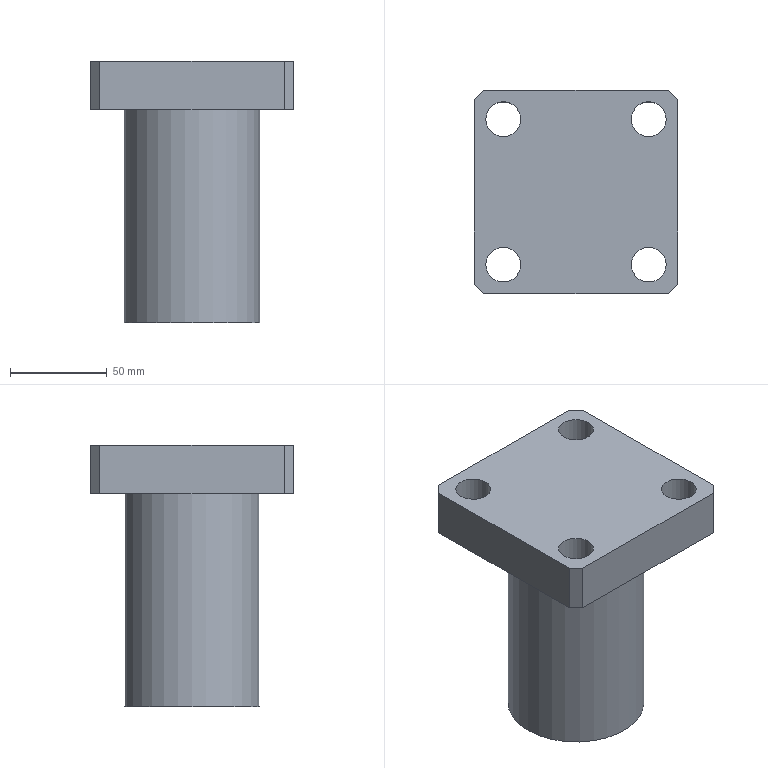Part | NX | features solid 2 | 1 solid | 16 faces | box 105 x 105 x 135 mm | volume 672258 mm3 | plane 11 | cylinder 5 | commonest cylinder face diameters 18 x4 70 x1
STEP:
#1=CARTESIAN_POINT('',(-237.5,207.5,100.));
#2=VERTEX_POINT('',#1);
#3=CARTESIAN_POINT('',(-237.5,112.5,100.));
#4=VERTEX_POINT('',#3);
#5=CARTESIAN_POINT('',(-237.5,210.,100.));
#6=DIRECTION('',(0.,-1.,0.));
#7=VECTOR('',#6,1000.);
#8=LINE('',#5,#7);
#9=EDGE_CURVE('',#2,#4,#8,.T.);
#10=ORIENTED_EDGE('',*,*,#9,.F.);
#11=CARTESIAN_POINT('',(-237.5,207.5,75.));
#12=VERTEX_POINT('',#11);
#13=CARTESIAN_POINT('',(-237.5,207.5,90.));
#14=DIRECTION('',(0.,0.,-1.));
#15=VECTOR('',#14,1000.);
#16=LINE('',#13,#15);
#17=EDGE_CURVE('',#2,#12,#16,.T.);
#18=ORIENTED_EDGE('',*,*,#17,.T.);
#19=CARTESIAN_POINT('',(-237.5,112.5,75.));
#20=VERTEX_POINT('',#19);
#21=CARTESIAN_POINT('',(-237.5,210.,75.));
#22=DIRECTION('',(0.,-1.,0.));
#23=VECTOR('',#22,1000.);
#24=LINE('',#21,#23);
#25=EDGE_CURVE('',#12,#20,#24,.T.);
#26=ORIENTED_EDGE('',*,*,#25,.T.);
#27=CARTESIAN_POINT('',(-237.5,112.5,90.));
#28=DIRECTION('',(0.,0.,1.));
#29=VECTOR('',#28,1000.);
#30=LINE('',#27,#29);
#31=EDGE_CURVE('',#20,#4,#30,.T.);
#32=ORIENTED_EDGE('',*,*,#31,.T.);
#33=EDGE_LOOP('',(#10,#18,#26,#32));
#34=FACE_BOUND('',#33,.T.);
#35=CARTESIAN_POINT('',(-237.5,210.,90.));
#36=DIRECTION('',(1.,0.,0.));
#37=DIRECTION('',(0.,0.,-1.));
#38=AXIS2_PLACEMENT_3D('',#35,#36,#37);
#39=PLANE('',#38);
#40=ADVANCED_FACE('',(#34),#39,.F.);
#41=CARTESIAN_POINT('',(-132.5,207.5,100.));
#42=VERTEX_POINT('',#41);
#43=CARTESIAN_POINT('',(-132.5,112.5,100.));
#44=VERTEX_POINT('',#43);
#45=CARTESIAN_POINT('',(-132.5,210.,100.));
#46=DIRECTION('',(0.,-1.,0.));
#47=VECTOR('',#46,1000.);
#48=LINE('',#45,#47);
#49=EDGE_CURVE('',#42,#44,#48,.T.);
#50=ORIENTED_EDGE('',*,*,#49,.T.);
#51=CARTESIAN_POINT('',(-132.5,112.5,75.));
#52=VERTEX_POINT('',#51);
#53=CARTESIAN_POINT('',(-132.5,112.5,75.));
#54=DIRECTION('',(0.,0.,-1.));
#55=VECTOR('',#54,1000.);
#56=LINE('',#53,#55);
#57=EDGE_CURVE('',#44,#52,#56,.T.);
#58=ORIENTED_EDGE('',*,*,#57,.T.);
#59=CARTESIAN_POINT('',(-132.5,207.5,75.));
#60=VERTEX_POINT('',#59);
#61=CARTESIAN_POINT('',(-132.5,210.,75.));
#62=DIRECTION('',(0.,-1.,0.));
#63=VECTOR('',#62,1000.);
#64=LINE('',#61,#63);
#65=EDGE_CURVE('',#60,#52,#64,.T.);
#66=ORIENTED_EDGE('',*,*,#65,.F.);
#67=CARTESIAN_POINT('',(-132.5,207.5,100.));
#68=DIRECTION('',(0.,0.,1.));
#69=VECTOR('',#68,1000.);
#70=LINE('',#67,#69);
#71=EDGE_CURVE('',#60,#42,#70,.T.);
#72=ORIENTED_EDGE('',*,*,#71,.T.);
#73=EDGE_LOOP('',(#50,#58,#66,#72));
#74=FACE_BOUND('',#73,.T.);
#75=CARTESIAN_POINT('',(-132.5,210.,90.));
#76=DIRECTION('',(1.,0.,0.));
#77=DIRECTION('',(0.,0.,-1.));
#78=AXIS2_PLACEMENT_3D('',#75,#76,#77);
#79=PLANE('',#78);
#80=ADVANCED_FACE('',(#74),#79,.T.);
#81=CARTESIAN_POINT('',(-137.5,212.5,100.));
#82=VERTEX_POINT('',#81);
#83=CARTESIAN_POINT('',(-232.5,212.5,100.));
#84=VERTEX_POINT('',#83);
#85=CARTESIAN_POINT('',(-185.,212.5,100.));
#86=DIRECTION('',(-1.,0.,0.));
#87=VECTOR('',#86,1000.);
#88=LINE('',#85,#87);
#89=EDGE_CURVE('',#82,#84,#88,.T.);
#90=ORIENTED_EDGE('',*,*,#89,.F.);
#91=CARTESIAN_POINT('',(-137.5,212.5,75.));
#92=VERTEX_POINT('',#91);
#93=CARTESIAN_POINT('',(-137.5,212.5,75.));
#94=DIRECTION('',(0.,0.,-1.));
#95=VECTOR('',#94,1000.);
#96=LINE('',#93,#95);
#97=EDGE_CURVE('',#82,#92,#96,.T.);
#98=ORIENTED_EDGE('',*,*,#97,.T.);
#99=CARTESIAN_POINT('',(-232.5,212.5,75.));
#100=VERTEX_POINT('',#99);
#101=CARTESIAN_POINT('',(-185.,212.5,75.));
#102=DIRECTION('',(-1.,0.,0.));
#103=VECTOR('',#102,1000.);
#104=LINE('',#101,#103);
#105=EDGE_CURVE('',#92,#100,#104,.T.);
#106=ORIENTED_EDGE('',*,*,#105,.T.);
#107=CARTESIAN_POINT('',(-232.5,212.5,90.));
#108=DIRECTION('',(0.,0.,1.));
#109=VECTOR('',#108,1000.);
#110=LINE('',#107,#109);
#111=EDGE_CURVE('',#100,#84,#110,.T.);
#112=ORIENTED_EDGE('',*,*,#111,.T.);
#113=EDGE_LOOP('',(#90,#98,#106,#112));
#114=FACE_BOUND('',#113,.T.);
#115=CARTESIAN_POINT('',(-185.,212.5,90.));
#116=DIRECTION('',(0.,-1.,0.));
#117=DIRECTION('',(0.,0.,-1.));
#118=AXIS2_PLACEMENT_3D('',#115,#116,#117);
#119=PLANE('',#118);
#120=ADVANCED_FACE('',(#114),#119,.F.);
#121=CARTESIAN_POINT('',(-232.5,107.5,75.));
#122=VERTEX_POINT('',#121);
#123=CARTESIAN_POINT('',(-137.5,107.5,75.));
#124=VERTEX_POINT('',#123);
#125=CARTESIAN_POINT('',(-185.,107.5,75.));
#126=DIRECTION('',(-1.,0.,0.));
#127=VECTOR('',#126,1000.);
#128=LINE('',#125,#127);
#129=EDGE_CURVE('',#122,#124,#128,.F.);
#130=ORIENTED_EDGE('',*,*,#129,.T.);
#131=CARTESIAN_POINT('',(-137.5,107.5,100.));
#132=VERTEX_POINT('',#131);
#133=CARTESIAN_POINT('',(-137.5,107.5,100.));
#134=DIRECTION('',(0.,0.,-1.));
#135=VECTOR('',#134,1000.);
#136=LINE('',#133,#135);
#137=EDGE_CURVE('',#124,#132,#136,.F.);
#138=ORIENTED_EDGE('',*,*,#137,.T.);
#139=CARTESIAN_POINT('',(-232.5,107.5,100.));
#140=VERTEX_POINT('',#139);
#141=CARTESIAN_POINT('',(-185.,107.5,100.));
#142=DIRECTION('',(1.,0.,0.));
#143=VECTOR('',#142,1000.);
#144=LINE('',#141,#143);
#145=EDGE_CURVE('',#132,#140,#144,.F.);
#146=ORIENTED_EDGE('',*,*,#145,.T.);
#147=CARTESIAN_POINT('',(-232.5,107.5,90.));
#148=DIRECTION('',(0.,0.,1.));
#149=VECTOR('',#148,1000.);
#150=LINE('',#147,#149);
#151=EDGE_CURVE('',#140,#122,#150,.F.);
#152=ORIENTED_EDGE('',*,*,#151,.T.);
#153=EDGE_LOOP('',(#130,#138,#146,#152));
#154=FACE_BOUND('',#153,.T.);
#155=CARTESIAN_POINT('',(-185.,107.5,90.));
#156=DIRECTION('',(0.,-1.,0.));
#157=DIRECTION('',(0.,0.,-1.));
#158=AXIS2_PLACEMENT_3D('',#155,#156,#157);
#159=PLANE('',#158);
#160=ADVANCED_FACE('',(#154),#159,.T.);
#161=CARTESIAN_POINT('',(-138.5,122.5,75.));
#162=VERTEX_POINT('',#161);
#163=CARTESIAN_POINT('',(-147.5,122.5,75.));
#164=DIRECTION('',(0.,0.,1.));
#165=DIRECTION('',(1.,0.,0.));
#166=AXIS2_PLACEMENT_3D('',#163,#164,#165);
#167=CIRCLE('',#166,9.);
#168=EDGE_CURVE('',#162,#162,#167,.F.);
#169=ORIENTED_EDGE('',*,*,#168,.T.);
#170=EDGE_LOOP('',(#169));
#171=FACE_BOUND('',#170,.T.);
#172=CARTESIAN_POINT('',(-138.5,122.5,100.));
#173=VERTEX_POINT('',#172);
#174=CARTESIAN_POINT('',(-147.5,122.5,100.));
#175=DIRECTION('',(0.,0.,1.));
#176=DIRECTION('',(1.,0.,0.));
#177=AXIS2_PLACEMENT_3D('',#174,#175,#176);
#178=CIRCLE('',#177,9.);
#179=EDGE_CURVE('',#173,#173,#178,.T.);
#180=ORIENTED_EDGE('',*,*,#179,.T.);
#181=EDGE_LOOP('',(#180));
#182=FACE_BOUND('',#181,.T.);
#183=CARTESIAN_POINT('',(-147.5,122.5,65.));
#184=DIRECTION('',(0.,0.,1.));
#185=DIRECTION('',(1.,0.,0.));
#186=AXIS2_PLACEMENT_3D('',#183,#184,#185);
#187=CYLINDRICAL_SURFACE('',#186,9.);
#188=ADVANCED_FACE('',(#171,#182),#187,.F.);
#189=CARTESIAN_POINT('',(-213.5,122.5,75.));
#190=VERTEX_POINT('',#189);
#191=CARTESIAN_POINT('',(-222.5,122.5,75.));
#192=DIRECTION('',(0.,0.,1.));
#193=DIRECTION('',(1.,0.,0.));
#194=AXIS2_PLACEMENT_3D('',#191,#192,#193);
#195=CIRCLE('',#194,9.);
#196=EDGE_CURVE('',#190,#190,#195,.F.);
#197=ORIENTED_EDGE('',*,*,#196,.T.);
#198=EDGE_LOOP('',(#197));
#199=FACE_BOUND('',#198,.T.);
#200=CARTESIAN_POINT('',(-213.5,122.5,100.));
#201=VERTEX_POINT('',#200);
#202=CARTESIAN_POINT('',(-222.5,122.5,100.));
#203=DIRECTION('',(0.,0.,1.));
#204=DIRECTION('',(1.,0.,0.));
#205=AXIS2_PLACEMENT_3D('',#202,#203,#204);
#206=CIRCLE('',#205,9.);
#207=EDGE_CURVE('',#201,#201,#206,.T.);
#208=ORIENTED_EDGE('',*,*,#207,.T.);
#209=EDGE_LOOP('',(#208));
#210=FACE_BOUND('',#209,.T.);
#211=CARTESIAN_POINT('',(-222.5,122.5,65.));
#212=DIRECTION('',(0.,0.,1.));
#213=DIRECTION('',(1.,0.,0.));
#214=AXIS2_PLACEMENT_3D('',#211,#212,#213);
#215=CYLINDRICAL_SURFACE('',#214,9.);
#216=ADVANCED_FACE('',(#199,#210),#215,.F.);
#217=CARTESIAN_POINT('',(-213.5,197.5,75.));
#218=VERTEX_POINT('',#217);
#219=CARTESIAN_POINT('',(-222.5,197.5,75.));
#220=DIRECTION('',(0.,0.,1.));
#221=DIRECTION('',(1.,0.,0.));
#222=AXIS2_PLACEMENT_3D('',#219,#220,#221);
#223=CIRCLE('',#222,9.);
#224=EDGE_CURVE('',#218,#218,#223,.F.);
#225=ORIENTED_EDGE('',*,*,#224,.T.);
#226=EDGE_LOOP('',(#225));
#227=FACE_BOUND('',#226,.T.);
#228=CARTESIAN_POINT('',(-213.5,197.5,100.));
#229=VERTEX_POINT('',#228);
#230=CARTESIAN_POINT('',(-222.5,197.5,100.));
#231=DIRECTION('',(0.,0.,1.));
#232=DIRECTION('',(1.,0.,0.));
#233=AXIS2_PLACEMENT_3D('',#230,#231,#232);
#234=CIRCLE('',#233,9.);
#235=EDGE_CURVE('',#229,#229,#234,.T.);
#236=ORIENTED_EDGE('',*,*,#235,.T.);
#237=EDGE_LOOP('',(#236));
#238=FACE_BOUND('',#237,.T.);
#239=CARTESIAN_POINT('',(-222.5,197.5,65.));
#240=DIRECTION('',(0.,0.,1.));
#241=DIRECTION('',(1.,0.,0.));
#242=AXIS2_PLACEMENT_3D('',#239,#240,#241);
#243=CYLINDRICAL_SURFACE('',#242,9.);
#244=ADVANCED_FACE('',(#227,#238),#243,.F.);
#245=CARTESIAN_POINT('',(-138.5,197.5,100.));
#246=VERTEX_POINT('',#245);
#247=CARTESIAN_POINT('',(-147.5,197.5,100.));
#248=DIRECTION('',(0.,0.,1.));
#249=DIRECTION('',(1.,0.,0.));
#250=AXIS2_PLACEMENT_3D('',#247,#248,#249);
#251=CIRCLE('',#250,9.);
#252=EDGE_CURVE('',#246,#246,#251,.T.);
#253=ORIENTED_EDGE('',*,*,#252,.F.);
#254=EDGE_LOOP('',(#253));
#255=FACE_BOUND('',#254,.T.);
#256=ORIENTED_EDGE('',*,*,#235,.F.);
#257=EDGE_LOOP('',(#256));
#258=FACE_BOUND('',#257,.T.);
#259=ORIENTED_EDGE('',*,*,#207,.F.);
#260=EDGE_LOOP('',(#259));
#261=FACE_BOUND('',#260,.T.);
#262=ORIENTED_EDGE('',*,*,#179,.F.);
#263=EDGE_LOOP('',(#262));
#264=FACE_BOUND('',#263,.T.);
#265=ORIENTED_EDGE('',*,*,#145,.F.);
#266=CARTESIAN_POINT('',(-135.,110.,100.));
#267=DIRECTION('',(-0.7071,-0.7071,0.));
#268=VECTOR('',#267,1000.);
#269=LINE('',#266,#268);
#270=EDGE_CURVE('',#132,#44,#269,.F.);
#271=ORIENTED_EDGE('',*,*,#270,.T.);
#272=ORIENTED_EDGE('',*,*,#49,.F.);
#273=CARTESIAN_POINT('',(-135.,210.,100.));
#274=DIRECTION('',(-0.7071,0.7071,0.));
#275=VECTOR('',#274,1000.);
#276=LINE('',#273,#275);
#277=EDGE_CURVE('',#42,#82,#276,.T.);
#278=ORIENTED_EDGE('',*,*,#277,.T.);
#279=ORIENTED_EDGE('',*,*,#89,.T.);
#280=CARTESIAN_POINT('',(-235.,210.,100.));
#281=DIRECTION('',(0.7071,0.7071,0.));
#282=VECTOR('',#281,1000.);
#283=LINE('',#280,#282);
#284=EDGE_CURVE('',#84,#2,#283,.F.);
#285=ORIENTED_EDGE('',*,*,#284,.T.);
#286=ORIENTED_EDGE('',*,*,#9,.T.);
#287=CARTESIAN_POINT('',(-235.,110.,100.));
#288=DIRECTION('',(0.7071,-0.7071,0.));
#289=VECTOR('',#288,1000.);
#290=LINE('',#287,#289);
#291=EDGE_CURVE('',#4,#140,#290,.T.);
#292=ORIENTED_EDGE('',*,*,#291,.T.);
#293=EDGE_LOOP('',(#265,#271,#272,#278,#279,#285,#286,#292));
#294=FACE_BOUND('',#293,.T.);
#295=CARTESIAN_POINT('',(-185.,160.,100.));
#296=DIRECTION('',(0.,0.,1.));
#297=DIRECTION('',(1.,0.,0.));
#298=AXIS2_PLACEMENT_3D('',#295,#296,#297);
#299=PLANE('',#298);
#300=ADVANCED_FACE('',(#255,#258,#261,#264,#294),#299,.T.);
#301=CARTESIAN_POINT('',(-138.5,197.5,75.));
#302=VERTEX_POINT('',#301);
#303=CARTESIAN_POINT('',(-147.5,197.5,75.));
#304=DIRECTION('',(0.,0.,1.));
#305=DIRECTION('',(1.,0.,0.));
#306=AXIS2_PLACEMENT_3D('',#303,#304,#305);
#307=CIRCLE('',#306,9.);
#308=EDGE_CURVE('',#302,#302,#307,.F.);
#309=ORIENTED_EDGE('',*,*,#308,.T.);
#310=EDGE_LOOP('',(#309));
#311=FACE_BOUND('',#310,.T.);
#312=ORIENTED_EDGE('',*,*,#252,.T.);
#313=EDGE_LOOP('',(#312));
#314=FACE_BOUND('',#313,.T.);
#315=CARTESIAN_POINT('',(-147.5,197.5,65.));
#316=DIRECTION('',(0.,0.,1.));
#317=DIRECTION('',(1.,0.,0.));
#318=AXIS2_PLACEMENT_3D('',#315,#316,#317);
#319=CYLINDRICAL_SURFACE('',#318,9.);
#320=ADVANCED_FACE('',(#311,#314),#319,.F.);
#321=CARTESIAN_POINT('',(-150.,160.,75.));
#322=VERTEX_POINT('',#321);
#323=CARTESIAN_POINT('',(-185.,160.,75.));
#324=DIRECTION('',(0.,0.,1.));
#325=DIRECTION('',(1.,0.,0.));
#326=AXIS2_PLACEMENT_3D('',#323,#324,#325);
#327=CIRCLE('',#326,35.);
#328=EDGE_CURVE('',#322,#322,#327,.F.);
#329=ORIENTED_EDGE('',*,*,#328,.F.);
#330=EDGE_LOOP('',(#329));
#331=FACE_BOUND('',#330,.T.);
#332=ORIENTED_EDGE('',*,*,#168,.F.);
#333=EDGE_LOOP('',(#332));
#334=FACE_BOUND('',#333,.T.);
#335=ORIENTED_EDGE('',*,*,#224,.F.);
#336=EDGE_LOOP('',(#335));
#337=FACE_BOUND('',#336,.T.);
#338=ORIENTED_EDGE('',*,*,#308,.F.);
#339=EDGE_LOOP('',(#338));
#340=FACE_BOUND('',#339,.T.);
#341=ORIENTED_EDGE('',*,*,#196,.F.);
#342=EDGE_LOOP('',(#341));
#343=FACE_BOUND('',#342,.T.);
#344=ORIENTED_EDGE('',*,*,#65,.T.);
#345=CARTESIAN_POINT('',(-132.5,112.5,75.));
#346=DIRECTION('',(0.7071,0.7071,0.));
#347=VECTOR('',#346,1000.);
#348=LINE('',#345,#347);
#349=EDGE_CURVE('',#52,#124,#348,.F.);
#350=ORIENTED_EDGE('',*,*,#349,.T.);
#351=ORIENTED_EDGE('',*,*,#129,.F.);
#352=CARTESIAN_POINT('',(-237.5,112.5,75.));
#353=DIRECTION('',(-0.7071,0.7071,0.));
#354=VECTOR('',#353,1000.);
#355=LINE('',#352,#354);
#356=EDGE_CURVE('',#122,#20,#355,.T.);
#357=ORIENTED_EDGE('',*,*,#356,.T.);
#358=ORIENTED_EDGE('',*,*,#25,.F.);
#359=CARTESIAN_POINT('',(-232.5,212.5,75.));
#360=DIRECTION('',(-0.7071,-0.7071,0.));
#361=VECTOR('',#360,1000.);
#362=LINE('',#359,#361);
#363=EDGE_CURVE('',#12,#100,#362,.F.);
#364=ORIENTED_EDGE('',*,*,#363,.T.);
#365=ORIENTED_EDGE('',*,*,#105,.F.);
#366=CARTESIAN_POINT('',(-137.5,212.5,75.));
#367=DIRECTION('',(0.7071,-0.7071,0.));
#368=VECTOR('',#367,1000.);
#369=LINE('',#366,#368);
#370=EDGE_CURVE('',#92,#60,#369,.T.);
#371=ORIENTED_EDGE('',*,*,#370,.T.);
#372=EDGE_LOOP('',(#344,#350,#351,#357,#358,#364,#365,#371));
#373=FACE_BOUND('',#372,.T.);
#374=CARTESIAN_POINT('',(105.,-110.,75.));
#375=DIRECTION('',(0.,0.,1.));
#376=DIRECTION('',(1.,0.,0.));
#377=AXIS2_PLACEMENT_3D('',#374,#375,#376);
#378=PLANE('',#377);
#379=ADVANCED_FACE('',(#331,#334,#337,#340,#343,#373),#378,.F.);
#380=ORIENTED_EDGE('',*,*,#270,.F.);
#381=ORIENTED_EDGE('',*,*,#137,.F.);
#382=ORIENTED_EDGE('',*,*,#349,.F.);
#383=ORIENTED_EDGE('',*,*,#57,.F.);
#384=EDGE_LOOP('',(#380,#381,#382,#383));
#385=FACE_BOUND('',#384,.T.);
#386=CARTESIAN_POINT('',(-132.5,112.5,90.));
#387=DIRECTION('',(-0.7071,0.7071,0.));
#388=DIRECTION('',(-0.7071,-0.7071,0.));
#389=AXIS2_PLACEMENT_3D('',#386,#387,#388);
#390=PLANE('',#389);
#391=ADVANCED_FACE('',(#385),#390,.F.);
#392=ORIENTED_EDGE('',*,*,#277,.F.);
#393=ORIENTED_EDGE('',*,*,#71,.F.);
#394=ORIENTED_EDGE('',*,*,#370,.F.);
#395=ORIENTED_EDGE('',*,*,#97,.F.);
#396=EDGE_LOOP('',(#392,#393,#394,#395));
#397=FACE_BOUND('',#396,.T.);
#398=CARTESIAN_POINT('',(-137.5,212.5,90.));
#399=DIRECTION('',(0.7071,0.7071,0.));
#400=DIRECTION('',(-0.7071,0.7071,0.));
#401=AXIS2_PLACEMENT_3D('',#398,#399,#400);
#402=PLANE('',#401);
#403=ADVANCED_FACE('',(#397),#402,.T.);
#404=ORIENTED_EDGE('',*,*,#363,.F.);
#405=ORIENTED_EDGE('',*,*,#17,.F.);
#406=ORIENTED_EDGE('',*,*,#284,.F.);
#407=ORIENTED_EDGE('',*,*,#111,.F.);
#408=EDGE_LOOP('',(#404,#405,#406,#407));
#409=FACE_BOUND('',#408,.T.);
#410=CARTESIAN_POINT('',(-232.5,212.5,90.));
#411=DIRECTION('',(0.7071,-0.7071,0.));
#412=DIRECTION('',(0.7071,0.7071,0.));
#413=AXIS2_PLACEMENT_3D('',#410,#411,#412);
#414=PLANE('',#413);
#415=ADVANCED_FACE('',(#409),#414,.F.);
#416=ORIENTED_EDGE('',*,*,#356,.F.);
#417=ORIENTED_EDGE('',*,*,#151,.F.);
#418=ORIENTED_EDGE('',*,*,#291,.F.);
#419=ORIENTED_EDGE('',*,*,#31,.F.);
#420=EDGE_LOOP('',(#416,#417,#418,#419));
#421=FACE_BOUND('',#420,.T.);
#422=CARTESIAN_POINT('',(-237.5,112.5,90.));
#423=DIRECTION('',(-0.7071,-0.7071,0.));
#424=DIRECTION('',(0.7071,-0.7071,0.));
#425=AXIS2_PLACEMENT_3D('',#422,#423,#424);
#426=PLANE('',#425);
#427=ADVANCED_FACE('',(#421),#426,.T.);
#428=CARTESIAN_POINT('',(-150.,160.,-35.));
#429=VERTEX_POINT('',#428);
#430=CARTESIAN_POINT('',(-185.,160.,-35.));
#431=DIRECTION('',(0.,0.,1.));
#432=DIRECTION('',(1.,0.,0.));
#433=AXIS2_PLACEMENT_3D('',#430,#431,#432);
#434=CIRCLE('',#433,35.);
#435=EDGE_CURVE('',#429,#429,#434,.F.);
#436=ORIENTED_EDGE('',*,*,#435,.F.);
#437=EDGE_LOOP('',(#436));
#438=FACE_BOUND('',#437,.T.);
#439=ORIENTED_EDGE('',*,*,#328,.T.);
#440=EDGE_LOOP('',(#439));
#441=FACE_BOUND('',#440,.T.);
#442=CARTESIAN_POINT('',(-185.,160.,-80.));
#443=DIRECTION('',(0.,0.,1.));
#444=DIRECTION('',(1.,0.,0.));
#445=AXIS2_PLACEMENT_3D('',#442,#443,#444);
#446=CYLINDRICAL_SURFACE('',#445,35.);
#447=ADVANCED_FACE('',(#438,#441),#446,.T.);
#448=ORIENTED_EDGE('',*,*,#435,.T.);
#449=EDGE_LOOP('',(#448));
#450=FACE_BOUND('',#449,.T.);
#451=CARTESIAN_POINT('',(-185.,160.,-35.));
#452=DIRECTION('',(0.,0.,1.));
#453=DIRECTION('',(1.,0.,0.));
#454=AXIS2_PLACEMENT_3D('',#451,#452,#453);
#455=PLANE('',#454);
#456=ADVANCED_FACE('',(#450),#455,.F.);
#457=CLOSED_SHELL('',(#40,#80,#120,#160,#188,#216,#244,#300,#320,#379,#391,#403,#415,#427,#447,#456));
#458=MANIFOLD_SOLID_BREP('',#457);
#459=(LENGTH_UNIT()NAMED_UNIT(*)SI_UNIT(.MILLI.,.METRE.));
#460=UNCERTAINTY_MEASURE_WITH_UNIT(LENGTH_MEASURE(0.00001),#459,'','');
#461=(NAMED_UNIT(*)PLANE_ANGLE_UNIT()SI_UNIT($,.RADIAN.));
#462=(NAMED_UNIT(*)SI_UNIT($,.STERADIAN.)SOLID_ANGLE_UNIT());
#463=(GEOMETRIC_REPRESENTATION_CONTEXT(3)GLOBAL_UNCERTAINTY_ASSIGNED_CONTEXT((#460))GLOBAL_UNIT_ASSIGNED_CONTEXT((#459,#461,#462))REPRESENTATION_CONTEXT('',''));
#464=ADVANCED_BREP_SHAPE_REPRESENTATION('',(#458),#463);